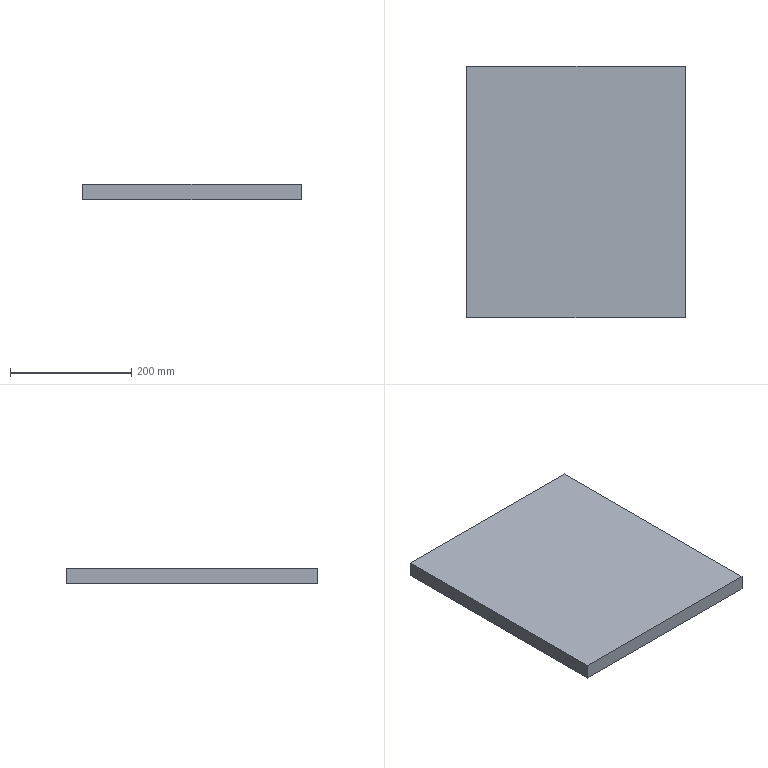Part | SolidWorks | features Extrusion 1 | 1 solid | 6 faces | box 360 x 415 x 25 mm | volume 3735000 mm3 | plane 6
STEP:
#1=CARTESIAN_POINT('',(0.,0.,0.));
#2=VERTEX_POINT('',#1);
#3=CARTESIAN_POINT('',(0.,-415.,0.));
#4=VERTEX_POINT('',#3);
#5=CARTESIAN_POINT('',(0.,0.,0.));
#6=DIRECTION('',(0.,-1.,0.));
#7=VECTOR('',#6,1000.);
#8=LINE('',#5,#7);
#9=EDGE_CURVE('',#2,#4,#8,.T.);
#10=ORIENTED_EDGE('',*,*,#9,.T.);
#11=CARTESIAN_POINT('',(0.,-415.,25.));
#12=VERTEX_POINT('',#11);
#13=CARTESIAN_POINT('',(0.,-415.,25.));
#14=DIRECTION('',(0.,0.,-1.));
#15=VECTOR('',#14,1000.);
#16=LINE('',#13,#15);
#17=EDGE_CURVE('',#12,#4,#16,.T.);
#18=ORIENTED_EDGE('',*,*,#17,.F.);
#19=CARTESIAN_POINT('',(0.,0.,25.));
#20=VERTEX_POINT('',#19);
#21=CARTESIAN_POINT('',(0.,0.,25.));
#22=DIRECTION('',(0.,-1.,0.));
#23=VECTOR('',#22,1000.);
#24=LINE('',#21,#23);
#25=EDGE_CURVE('',#20,#12,#24,.T.);
#26=ORIENTED_EDGE('',*,*,#25,.F.);
#27=CARTESIAN_POINT('',(0.,0.,25.));
#28=DIRECTION('',(0.,0.,-1.));
#29=VECTOR('',#28,1000.);
#30=LINE('',#27,#29);
#31=EDGE_CURVE('',#20,#2,#30,.T.);
#32=ORIENTED_EDGE('',*,*,#31,.T.);
#33=EDGE_LOOP('',(#10,#18,#26,#32));
#34=FACE_OUTER_BOUND('',#33,.T.);
#35=CARTESIAN_POINT('',(0.,0.,25.));
#36=DIRECTION('',(1.,0.,0.));
#37=DIRECTION('',(0.,1.,0.));
#38=AXIS2_PLACEMENT_3D('',#35,#36,#37);
#39=PLANE('',#38);
#40=ADVANCED_FACE('',(#34),#39,.F.);
#41=CARTESIAN_POINT('',(360.,-415.,0.));
#42=VERTEX_POINT('',#41);
#43=CARTESIAN_POINT('',(0.,-415.,0.));
#44=DIRECTION('',(1.,0.,0.));
#45=VECTOR('',#44,1000.);
#46=LINE('',#43,#45);
#47=EDGE_CURVE('',#4,#42,#46,.T.);
#48=ORIENTED_EDGE('',*,*,#47,.T.);
#49=CARTESIAN_POINT('',(360.,-415.,25.));
#50=VERTEX_POINT('',#49);
#51=CARTESIAN_POINT('',(360.,-415.,25.));
#52=DIRECTION('',(0.,0.,-1.));
#53=VECTOR('',#52,1000.);
#54=LINE('',#51,#53);
#55=EDGE_CURVE('',#50,#42,#54,.T.);
#56=ORIENTED_EDGE('',*,*,#55,.F.);
#57=CARTESIAN_POINT('',(0.,-415.,25.));
#58=DIRECTION('',(1.,0.,0.));
#59=VECTOR('',#58,1000.);
#60=LINE('',#57,#59);
#61=EDGE_CURVE('',#12,#50,#60,.T.);
#62=ORIENTED_EDGE('',*,*,#61,.F.);
#63=ORIENTED_EDGE('',*,*,#17,.T.);
#64=EDGE_LOOP('',(#48,#56,#62,#63));
#65=FACE_OUTER_BOUND('',#64,.T.);
#66=CARTESIAN_POINT('',(0.,-415.,25.));
#67=DIRECTION('',(0.,1.,0.));
#68=DIRECTION('',(0.,0.,1.));
#69=AXIS2_PLACEMENT_3D('',#66,#67,#68);
#70=PLANE('',#69);
#71=ADVANCED_FACE('',(#65),#70,.F.);
#72=CARTESIAN_POINT('',(360.,0.,0.));
#73=VERTEX_POINT('',#72);
#74=CARTESIAN_POINT('',(360.,0.,0.));
#75=DIRECTION('',(0.,1.,0.));
#76=VECTOR('',#75,1000.);
#77=LINE('',#74,#76);
#78=EDGE_CURVE('',#42,#73,#77,.T.);
#79=ORIENTED_EDGE('',*,*,#78,.T.);
#80=CARTESIAN_POINT('',(360.,0.,25.));
#81=VERTEX_POINT('',#80);
#82=CARTESIAN_POINT('',(360.,0.,25.));
#83=DIRECTION('',(0.,0.,-1.));
#84=VECTOR('',#83,1000.);
#85=LINE('',#82,#84);
#86=EDGE_CURVE('',#81,#73,#85,.T.);
#87=ORIENTED_EDGE('',*,*,#86,.F.);
#88=CARTESIAN_POINT('',(360.,0.,25.));
#89=DIRECTION('',(0.,1.,0.));
#90=VECTOR('',#89,1000.);
#91=LINE('',#88,#90);
#92=EDGE_CURVE('',#50,#81,#91,.T.);
#93=ORIENTED_EDGE('',*,*,#92,.F.);
#94=ORIENTED_EDGE('',*,*,#55,.T.);
#95=EDGE_LOOP('',(#79,#87,#93,#94));
#96=FACE_OUTER_BOUND('',#95,.T.);
#97=CARTESIAN_POINT('',(360.,0.,25.));
#98=DIRECTION('',(-1.,0.,0.));
#99=DIRECTION('',(0.,-1.,0.));
#100=AXIS2_PLACEMENT_3D('',#97,#98,#99);
#101=PLANE('',#100);
#102=ADVANCED_FACE('',(#96),#101,.F.);
#103=CARTESIAN_POINT('',(0.,0.,0.));
#104=DIRECTION('',(-1.,0.,0.));
#105=VECTOR('',#104,1000.);
#106=LINE('',#103,#105);
#107=EDGE_CURVE('',#73,#2,#106,.T.);
#108=ORIENTED_EDGE('',*,*,#107,.T.);
#109=ORIENTED_EDGE('',*,*,#31,.F.);
#110=CARTESIAN_POINT('',(0.,0.,25.));
#111=DIRECTION('',(-1.,0.,0.));
#112=VECTOR('',#111,1000.);
#113=LINE('',#110,#112);
#114=EDGE_CURVE('',#81,#20,#113,.T.);
#115=ORIENTED_EDGE('',*,*,#114,.F.);
#116=ORIENTED_EDGE('',*,*,#86,.T.);
#117=EDGE_LOOP('',(#108,#109,#115,#116));
#118=FACE_OUTER_BOUND('',#117,.T.);
#119=CARTESIAN_POINT('',(0.,0.,25.));
#120=DIRECTION('',(0.,-1.,0.));
#121=DIRECTION('',(0.,0.,-1.));
#122=AXIS2_PLACEMENT_3D('',#119,#120,#121);
#123=PLANE('',#122);
#124=ADVANCED_FACE('',(#118),#123,.F.);
#125=ORIENTED_EDGE('',*,*,#25,.T.);
#126=ORIENTED_EDGE('',*,*,#61,.T.);
#127=ORIENTED_EDGE('',*,*,#92,.T.);
#128=ORIENTED_EDGE('',*,*,#114,.T.);
#129=EDGE_LOOP('',(#125,#126,#127,#128));
#130=FACE_OUTER_BOUND('',#129,.T.);
#131=CARTESIAN_POINT('',(0.,0.,25.));
#132=DIRECTION('',(0.,0.,1.));
#133=DIRECTION('',(1.,0.,0.));
#134=AXIS2_PLACEMENT_3D('',#131,#132,#133);
#135=PLANE('',#134);
#136=ADVANCED_FACE('',(#130),#135,.T.);
#137=ORIENTED_EDGE('',*,*,#9,.F.);
#138=ORIENTED_EDGE('',*,*,#107,.F.);
#139=ORIENTED_EDGE('',*,*,#78,.F.);
#140=ORIENTED_EDGE('',*,*,#47,.F.);
#141=EDGE_LOOP('',(#137,#138,#139,#140));
#142=FACE_OUTER_BOUND('',#141,.T.);
#143=CARTESIAN_POINT('',(0.,0.,0.));
#144=DIRECTION('',(0.,0.,1.));
#145=DIRECTION('',(1.,0.,0.));
#146=AXIS2_PLACEMENT_3D('',#143,#144,#145);
#147=PLANE('',#146);
#148=ADVANCED_FACE('',(#142),#147,.F.);
#149=CLOSED_SHELL('',(#40,#71,#102,#124,#136,#148));
#150=MANIFOLD_SOLID_BREP('',#149);
#151=CARTESIAN_POINT('',(0.,0.,0.));
#152=DIRECTION('',(0.,0.,1.));
#153=DIRECTION('',(1.,0.,0.));
#154=AXIS2_PLACEMENT_3D('',#151,#152,#153);
#155=(LENGTH_UNIT()NAMED_UNIT(*)SI_UNIT(.MILLI.,.METRE.));
#156=UNCERTAINTY_MEASURE_WITH_UNIT(LENGTH_MEASURE(0.00001),#155,'','');
#157=(NAMED_UNIT(*)PLANE_ANGLE_UNIT()SI_UNIT($,.RADIAN.));
#158=(NAMED_UNIT(*)SI_UNIT($,.STERADIAN.)SOLID_ANGLE_UNIT());
#159=(GEOMETRIC_REPRESENTATION_CONTEXT(3)GLOBAL_UNCERTAINTY_ASSIGNED_CONTEXT((#156))GLOBAL_UNIT_ASSIGNED_CONTEXT((#155,#157,#158))REPRESENTATION_CONTEXT('',''));
#160=ADVANCED_BREP_SHAPE_REPRESENTATION('',(#150,#154),#159);